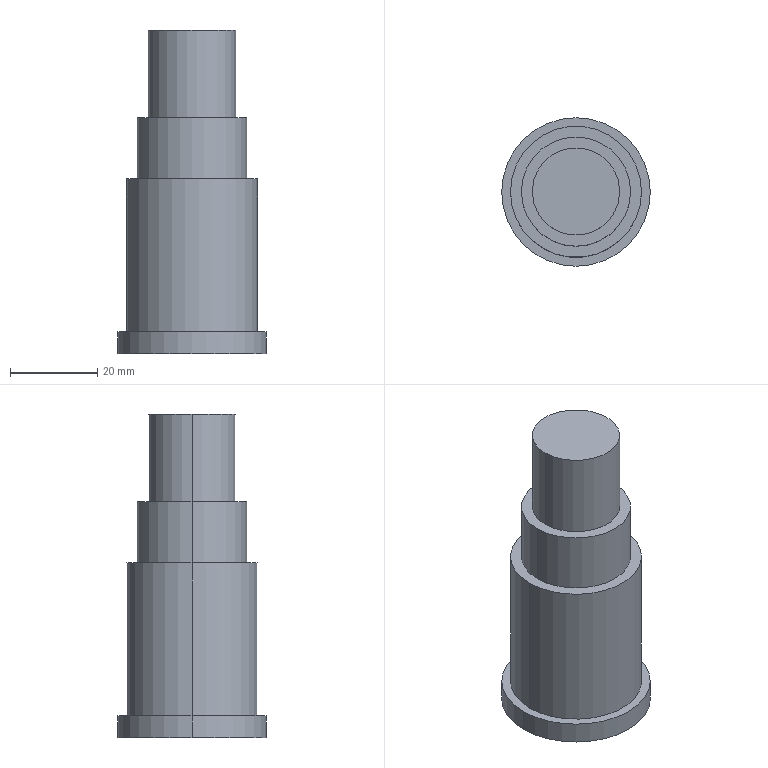Part | NX | features BREP 1 | 1 solid | 13 faces | box 34 x 34 x 74 mm | volume 42435 mm3 | cylinder 8 | plane 5 | commonest cylinder face diameters 20 x2 25 x2 30 x2 34 x2
STEP:
#1=CARTESIAN_POINT('',(15.,0.,-69.));
#2=VERTEX_POINT('',#1);
#3=CARTESIAN_POINT('',(-15.,0.,-69.));
#4=VERTEX_POINT('',#3);
#5=CARTESIAN_POINT('',(0.,0.,-69.));
#6=DIRECTION('',(0.,0.,1.));
#7=DIRECTION('',(1.,0.,0.));
#8=AXIS2_PLACEMENT_3D('',#5,#6,#7);
#9=CIRCLE('',#8,15.);
#10=EDGE_CURVE('',#2,#4,#9,.T.);
#11=ORIENTED_EDGE('',*,*,#10,.T.);
#12=CARTESIAN_POINT('',(-15.,0.,-34.));
#13=VERTEX_POINT('',#12);
#14=CARTESIAN_POINT('',(-15.,0.,-69.));
#15=DIRECTION('',(0.,0.,1.));
#16=VECTOR('',#15,1000.);
#17=LINE('',#14,#16);
#18=EDGE_CURVE('',#13,#4,#17,.F.);
#19=ORIENTED_EDGE('',*,*,#18,.F.);
#20=CARTESIAN_POINT('',(15.,0.,-34.));
#21=VERTEX_POINT('',#20);
#22=CARTESIAN_POINT('',(0.,0.,-34.));
#23=DIRECTION('',(0.,0.,-1.));
#24=DIRECTION('',(1.,0.,0.));
#25=AXIS2_PLACEMENT_3D('',#22,#23,#24);
#26=CIRCLE('',#25,15.);
#27=EDGE_CURVE('',#13,#21,#26,.T.);
#28=ORIENTED_EDGE('',*,*,#27,.T.);
#29=CARTESIAN_POINT('',(15.,0.,-69.));
#30=DIRECTION('',(0.,0.,1.));
#31=VECTOR('',#30,1000.);
#32=LINE('',#29,#31);
#33=EDGE_CURVE('',#21,#2,#32,.F.);
#34=ORIENTED_EDGE('',*,*,#33,.T.);
#35=EDGE_LOOP('',(#11,#19,#28,#34));
#36=FACE_BOUND('',#35,.T.);
#37=CARTESIAN_POINT('',(0.,0.,-69.));
#38=DIRECTION('',(0.,0.,1.));
#39=DIRECTION('',(1.,0.,0.));
#40=AXIS2_PLACEMENT_3D('',#37,#38,#39);
#41=CYLINDRICAL_SURFACE('',#40,15.);
#42=ADVANCED_FACE('',(#36),#41,.T.);
#43=CARTESIAN_POINT('',(12.5,0.,-34.));
#44=VERTEX_POINT('',#43);
#45=CARTESIAN_POINT('',(-12.5,0.,-34.));
#46=VERTEX_POINT('',#45);
#47=CARTESIAN_POINT('',(0.,0.,-34.));
#48=DIRECTION('',(0.,0.,1.));
#49=DIRECTION('',(1.,0.,0.));
#50=AXIS2_PLACEMENT_3D('',#47,#48,#49);
#51=CIRCLE('',#50,12.5);
#52=EDGE_CURVE('',#44,#46,#51,.T.);
#53=ORIENTED_EDGE('',*,*,#52,.T.);
#54=CARTESIAN_POINT('',(-12.5,0.,-20.));
#55=VERTEX_POINT('',#54);
#56=CARTESIAN_POINT('',(-12.5,0.,-34.));
#57=DIRECTION('',(0.,0.,1.));
#58=VECTOR('',#57,1000.);
#59=LINE('',#56,#58);
#60=EDGE_CURVE('',#55,#46,#59,.F.);
#61=ORIENTED_EDGE('',*,*,#60,.F.);
#62=CARTESIAN_POINT('',(12.5,0.,-20.));
#63=VERTEX_POINT('',#62);
#64=CARTESIAN_POINT('',(0.,0.,-20.));
#65=DIRECTION('',(0.,0.,-1.));
#66=DIRECTION('',(1.,0.,0.));
#67=AXIS2_PLACEMENT_3D('',#64,#65,#66);
#68=CIRCLE('',#67,12.5);
#69=EDGE_CURVE('',#55,#63,#68,.T.);
#70=ORIENTED_EDGE('',*,*,#69,.T.);
#71=CARTESIAN_POINT('',(12.5,0.,-34.));
#72=DIRECTION('',(0.,0.,1.));
#73=VECTOR('',#72,1000.);
#74=LINE('',#71,#73);
#75=EDGE_CURVE('',#63,#44,#74,.F.);
#76=ORIENTED_EDGE('',*,*,#75,.T.);
#77=EDGE_LOOP('',(#53,#61,#70,#76));
#78=FACE_BOUND('',#77,.T.);
#79=CARTESIAN_POINT('',(0.,0.,-34.));
#80=DIRECTION('',(0.,0.,1.));
#81=DIRECTION('',(1.,0.,0.));
#82=AXIS2_PLACEMENT_3D('',#79,#80,#81);
#83=CYLINDRICAL_SURFACE('',#82,12.5);
#84=ADVANCED_FACE('',(#78),#83,.T.);
#85=CARTESIAN_POINT('',(17.,0.,-74.));
#86=VERTEX_POINT('',#85);
#87=CARTESIAN_POINT('',(-17.,0.,-74.));
#88=VERTEX_POINT('',#87);
#89=CARTESIAN_POINT('',(0.,0.,-74.));
#90=DIRECTION('',(0.,0.,1.));
#91=DIRECTION('',(1.,0.,0.));
#92=AXIS2_PLACEMENT_3D('',#89,#90,#91);
#93=CIRCLE('',#92,17.);
#94=EDGE_CURVE('',#86,#88,#93,.T.);
#95=ORIENTED_EDGE('',*,*,#94,.T.);
#96=CARTESIAN_POINT('',(-17.,0.,-69.));
#97=VERTEX_POINT('',#96);
#98=CARTESIAN_POINT('',(-17.,0.,-74.));
#99=DIRECTION('',(0.,0.,1.));
#100=VECTOR('',#99,1000.);
#101=LINE('',#98,#100);
#102=EDGE_CURVE('',#97,#88,#101,.F.);
#103=ORIENTED_EDGE('',*,*,#102,.F.);
#104=CARTESIAN_POINT('',(17.,0.,-69.));
#105=VERTEX_POINT('',#104);
#106=CARTESIAN_POINT('',(0.,0.,-69.));
#107=DIRECTION('',(0.,0.,-1.));
#108=DIRECTION('',(1.,0.,0.));
#109=AXIS2_PLACEMENT_3D('',#106,#107,#108);
#110=CIRCLE('',#109,17.);
#111=EDGE_CURVE('',#97,#105,#110,.T.);
#112=ORIENTED_EDGE('',*,*,#111,.T.);
#113=CARTESIAN_POINT('',(17.,0.,-74.));
#114=DIRECTION('',(0.,0.,1.));
#115=VECTOR('',#114,1000.);
#116=LINE('',#113,#115);
#117=EDGE_CURVE('',#105,#86,#116,.F.);
#118=ORIENTED_EDGE('',*,*,#117,.T.);
#119=EDGE_LOOP('',(#95,#103,#112,#118));
#120=FACE_BOUND('',#119,.T.);
#121=CARTESIAN_POINT('',(0.,0.,-74.));
#122=DIRECTION('',(0.,0.,1.));
#123=DIRECTION('',(1.,0.,0.));
#124=AXIS2_PLACEMENT_3D('',#121,#122,#123);
#125=CYLINDRICAL_SURFACE('',#124,17.);
#126=ADVANCED_FACE('',(#120),#125,.T.);
#127=CARTESIAN_POINT('',(10.,0.,-20.));
#128=VERTEX_POINT('',#127);
#129=CARTESIAN_POINT('',(-10.,0.,-20.));
#130=VERTEX_POINT('',#129);
#131=CARTESIAN_POINT('',(0.,0.,-20.));
#132=DIRECTION('',(0.,0.,1.));
#133=DIRECTION('',(1.,0.,0.));
#134=AXIS2_PLACEMENT_3D('',#131,#132,#133);
#135=CIRCLE('',#134,10.);
#136=EDGE_CURVE('',#128,#130,#135,.T.);
#137=ORIENTED_EDGE('',*,*,#136,.T.);
#138=CARTESIAN_POINT('',(-10.,0.,0.));
#139=VERTEX_POINT('',#138);
#140=CARTESIAN_POINT('',(-10.,0.,-20.));
#141=DIRECTION('',(0.,0.,1.));
#142=VECTOR('',#141,1000.);
#143=LINE('',#140,#142);
#144=EDGE_CURVE('',#139,#130,#143,.F.);
#145=ORIENTED_EDGE('',*,*,#144,.F.);
#146=CARTESIAN_POINT('',(10.,0.,0.));
#147=VERTEX_POINT('',#146);
#148=CARTESIAN_POINT('',(0.,0.,0.));
#149=DIRECTION('',(0.,0.,-1.));
#150=DIRECTION('',(1.,0.,0.));
#151=AXIS2_PLACEMENT_3D('',#148,#149,#150);
#152=CIRCLE('',#151,10.);
#153=EDGE_CURVE('',#139,#147,#152,.T.);
#154=ORIENTED_EDGE('',*,*,#153,.T.);
#155=CARTESIAN_POINT('',(10.,0.,-20.));
#156=DIRECTION('',(0.,0.,1.));
#157=VECTOR('',#156,1000.);
#158=LINE('',#155,#157);
#159=EDGE_CURVE('',#147,#128,#158,.F.);
#160=ORIENTED_EDGE('',*,*,#159,.T.);
#161=EDGE_LOOP('',(#137,#145,#154,#160));
#162=FACE_BOUND('',#161,.T.);
#163=CARTESIAN_POINT('',(0.,0.,-20.));
#164=DIRECTION('',(0.,0.,1.));
#165=DIRECTION('',(1.,0.,0.));
#166=AXIS2_PLACEMENT_3D('',#163,#164,#165);
#167=CYLINDRICAL_SURFACE('',#166,10.);
#168=ADVANCED_FACE('',(#162),#167,.T.);
#169=ORIENTED_EDGE('',*,*,#18,.T.);
#170=CARTESIAN_POINT('',(0.,0.,-69.));
#171=DIRECTION('',(0.,0.,1.));
#172=DIRECTION('',(1.,0.,0.));
#173=AXIS2_PLACEMENT_3D('',#170,#171,#172);
#174=CIRCLE('',#173,15.);
#175=EDGE_CURVE('',#4,#2,#174,.T.);
#176=ORIENTED_EDGE('',*,*,#175,.T.);
#177=ORIENTED_EDGE('',*,*,#33,.F.);
#178=CARTESIAN_POINT('',(0.,0.,-34.));
#179=DIRECTION('',(0.,0.,-1.));
#180=DIRECTION('',(1.,0.,0.));
#181=AXIS2_PLACEMENT_3D('',#178,#179,#180);
#182=CIRCLE('',#181,15.);
#183=EDGE_CURVE('',#21,#13,#182,.T.);
#184=ORIENTED_EDGE('',*,*,#183,.T.);
#185=EDGE_LOOP('',(#169,#176,#177,#184));
#186=FACE_BOUND('',#185,.T.);
#187=CARTESIAN_POINT('',(0.,0.,-69.));
#188=DIRECTION('',(0.,0.,1.));
#189=DIRECTION('',(1.,0.,0.));
#190=AXIS2_PLACEMENT_3D('',#187,#188,#189);
#191=CYLINDRICAL_SURFACE('',#190,15.);
#192=ADVANCED_FACE('',(#186),#191,.T.);
#193=ORIENTED_EDGE('',*,*,#183,.F.);
#194=ORIENTED_EDGE('',*,*,#27,.F.);
#195=EDGE_LOOP('',(#193,#194));
#196=FACE_BOUND('',#195,.T.);
#197=ORIENTED_EDGE('',*,*,#52,.F.);
#198=CARTESIAN_POINT('',(0.,0.,-34.));
#199=DIRECTION('',(0.,0.,1.));
#200=DIRECTION('',(1.,0.,0.));
#201=AXIS2_PLACEMENT_3D('',#198,#199,#200);
#202=CIRCLE('',#201,12.5);
#203=EDGE_CURVE('',#46,#44,#202,.T.);
#204=ORIENTED_EDGE('',*,*,#203,.F.);
#205=EDGE_LOOP('',(#197,#204));
#206=FACE_BOUND('',#205,.T.);
#207=CARTESIAN_POINT('',(0.,0.,-34.));
#208=DIRECTION('',(0.,0.,-1.));
#209=DIRECTION('',(0.,-1.,0.));
#210=AXIS2_PLACEMENT_3D('',#207,#208,#209);
#211=PLANE('',#210);
#212=ADVANCED_FACE('',(#196,#206),#211,.F.);
#213=CARTESIAN_POINT('',(0.,0.,-69.));
#214=DIRECTION('',(0.,0.,-1.));
#215=DIRECTION('',(1.,0.,0.));
#216=AXIS2_PLACEMENT_3D('',#213,#214,#215);
#217=CIRCLE('',#216,17.);
#218=EDGE_CURVE('',#105,#97,#217,.T.);
#219=ORIENTED_EDGE('',*,*,#218,.F.);
#220=ORIENTED_EDGE('',*,*,#111,.F.);
#221=EDGE_LOOP('',(#219,#220));
#222=FACE_BOUND('',#221,.T.);
#223=ORIENTED_EDGE('',*,*,#10,.F.);
#224=ORIENTED_EDGE('',*,*,#175,.F.);
#225=EDGE_LOOP('',(#223,#224));
#226=FACE_BOUND('',#225,.T.);
#227=CARTESIAN_POINT('',(0.,0.,-69.));
#228=DIRECTION('',(0.,0.,-1.));
#229=DIRECTION('',(0.,-1.,0.));
#230=AXIS2_PLACEMENT_3D('',#227,#228,#229);
#231=PLANE('',#230);
#232=ADVANCED_FACE('',(#222,#226),#231,.F.);
#233=ORIENTED_EDGE('',*,*,#60,.T.);
#234=ORIENTED_EDGE('',*,*,#203,.T.);
#235=ORIENTED_EDGE('',*,*,#75,.F.);
#236=CARTESIAN_POINT('',(0.,0.,-20.));
#237=DIRECTION('',(0.,0.,-1.));
#238=DIRECTION('',(1.,0.,0.));
#239=AXIS2_PLACEMENT_3D('',#236,#237,#238);
#240=CIRCLE('',#239,12.5);
#241=EDGE_CURVE('',#63,#55,#240,.T.);
#242=ORIENTED_EDGE('',*,*,#241,.T.);
#243=EDGE_LOOP('',(#233,#234,#235,#242));
#244=FACE_BOUND('',#243,.T.);
#245=CARTESIAN_POINT('',(0.,0.,-34.));
#246=DIRECTION('',(0.,0.,1.));
#247=DIRECTION('',(1.,0.,0.));
#248=AXIS2_PLACEMENT_3D('',#245,#246,#247);
#249=CYLINDRICAL_SURFACE('',#248,12.5);
#250=ADVANCED_FACE('',(#244),#249,.T.);
#251=ORIENTED_EDGE('',*,*,#102,.T.);
#252=CARTESIAN_POINT('',(0.,0.,-74.));
#253=DIRECTION('',(0.,0.,1.));
#254=DIRECTION('',(1.,0.,0.));
#255=AXIS2_PLACEMENT_3D('',#252,#253,#254);
#256=CIRCLE('',#255,17.);
#257=EDGE_CURVE('',#88,#86,#256,.T.);
#258=ORIENTED_EDGE('',*,*,#257,.T.);
#259=ORIENTED_EDGE('',*,*,#117,.F.);
#260=ORIENTED_EDGE('',*,*,#218,.T.);
#261=EDGE_LOOP('',(#251,#258,#259,#260));
#262=FACE_BOUND('',#261,.T.);
#263=CARTESIAN_POINT('',(0.,0.,-74.));
#264=DIRECTION('',(0.,0.,1.));
#265=DIRECTION('',(1.,0.,0.));
#266=AXIS2_PLACEMENT_3D('',#263,#264,#265);
#267=CYLINDRICAL_SURFACE('',#266,17.);
#268=ADVANCED_FACE('',(#262),#267,.T.);
#269=ORIENTED_EDGE('',*,*,#241,.F.);
#270=ORIENTED_EDGE('',*,*,#69,.F.);
#271=EDGE_LOOP('',(#269,#270));
#272=FACE_BOUND('',#271,.T.);
#273=ORIENTED_EDGE('',*,*,#136,.F.);
#274=CARTESIAN_POINT('',(0.,0.,-20.));
#275=DIRECTION('',(0.,0.,1.));
#276=DIRECTION('',(1.,0.,0.));
#277=AXIS2_PLACEMENT_3D('',#274,#275,#276);
#278=CIRCLE('',#277,10.);
#279=EDGE_CURVE('',#130,#128,#278,.T.);
#280=ORIENTED_EDGE('',*,*,#279,.F.);
#281=EDGE_LOOP('',(#273,#280));
#282=FACE_BOUND('',#281,.T.);
#283=CARTESIAN_POINT('',(0.,0.,-20.));
#284=DIRECTION('',(0.,0.,-1.));
#285=DIRECTION('',(0.,-1.,0.));
#286=AXIS2_PLACEMENT_3D('',#283,#284,#285);
#287=PLANE('',#286);
#288=ADVANCED_FACE('',(#272,#282),#287,.F.);
#289=ORIENTED_EDGE('',*,*,#94,.F.);
#290=ORIENTED_EDGE('',*,*,#257,.F.);
#291=EDGE_LOOP('',(#289,#290));
#292=FACE_BOUND('',#291,.T.);
#293=CARTESIAN_POINT('',(0.,0.,-74.));
#294=DIRECTION('',(0.,0.,-1.));
#295=DIRECTION('',(0.,-1.,0.));
#296=AXIS2_PLACEMENT_3D('',#293,#294,#295);
#297=PLANE('',#296);
#298=ADVANCED_FACE('',(#292),#297,.T.);
#299=ORIENTED_EDGE('',*,*,#144,.T.);
#300=ORIENTED_EDGE('',*,*,#279,.T.);
#301=ORIENTED_EDGE('',*,*,#159,.F.);
#302=CARTESIAN_POINT('',(0.,0.,0.));
#303=DIRECTION('',(0.,0.,-1.));
#304=DIRECTION('',(1.,0.,0.));
#305=AXIS2_PLACEMENT_3D('',#302,#303,#304);
#306=CIRCLE('',#305,10.);
#307=EDGE_CURVE('',#147,#139,#306,.T.);
#308=ORIENTED_EDGE('',*,*,#307,.T.);
#309=EDGE_LOOP('',(#299,#300,#301,#308));
#310=FACE_BOUND('',#309,.T.);
#311=CARTESIAN_POINT('',(0.,0.,-20.));
#312=DIRECTION('',(0.,0.,1.));
#313=DIRECTION('',(1.,0.,0.));
#314=AXIS2_PLACEMENT_3D('',#311,#312,#313);
#315=CYLINDRICAL_SURFACE('',#314,10.);
#316=ADVANCED_FACE('',(#310),#315,.T.);
#317=ORIENTED_EDGE('',*,*,#307,.F.);
#318=ORIENTED_EDGE('',*,*,#153,.F.);
#319=EDGE_LOOP('',(#317,#318));
#320=FACE_BOUND('',#319,.T.);
#321=CARTESIAN_POINT('',(0.,0.,0.));
#322=DIRECTION('',(0.,0.,1.));
#323=DIRECTION('',(1.,0.,0.));
#324=AXIS2_PLACEMENT_3D('',#321,#322,#323);
#325=PLANE('',#324);
#326=ADVANCED_FACE('',(#320),#325,.T.);
#327=CLOSED_SHELL('',(#42,#84,#126,#168,#192,#212,#232,#250,#268,#288,#298,#316,#326));
#328=MANIFOLD_SOLID_BREP('',#327);
#329=(LENGTH_UNIT()NAMED_UNIT(*)SI_UNIT(.MILLI.,.METRE.));
#330=UNCERTAINTY_MEASURE_WITH_UNIT(LENGTH_MEASURE(0.00001),#329,'','');
#331=(NAMED_UNIT(*)PLANE_ANGLE_UNIT()SI_UNIT($,.RADIAN.));
#332=(NAMED_UNIT(*)SI_UNIT($,.STERADIAN.)SOLID_ANGLE_UNIT());
#333=(GEOMETRIC_REPRESENTATION_CONTEXT(3)GLOBAL_UNCERTAINTY_ASSIGNED_CONTEXT((#330))GLOBAL_UNIT_ASSIGNED_CONTEXT((#329,#331,#332))REPRESENTATION_CONTEXT('',''));
#334=ADVANCED_BREP_SHAPE_REPRESENTATION('',(#328),#333);